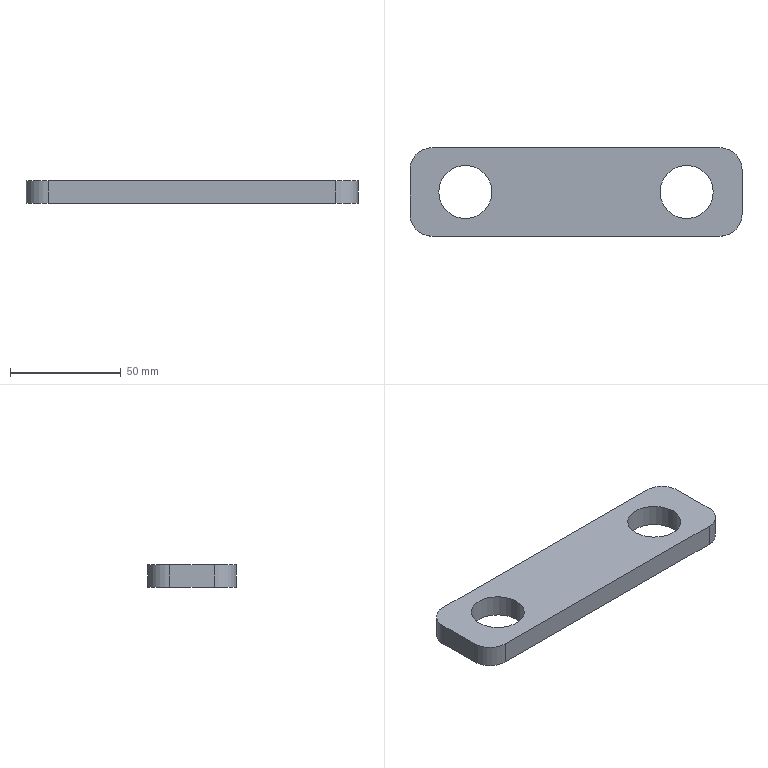Part | SolidWorks | features Extrusion 1, Fillet 1 | 1 solid | 14 faces | box 150 x 40 x 10 mm | volume 50094 mm3 | cylinder 8 | plane 6 | commonest cylinder face diameters 20 x4 24 x4
STEP:
#1=CARTESIAN_POINT('',(-62.,0.,10.));
#2=VERTEX_POINT('',#1);
#3=CARTESIAN_POINT('',(-38.,0.,10.));
#4=VERTEX_POINT('',#3);
#5=CARTESIAN_POINT('',(-50.,0.,10.));
#6=DIRECTION('',(0.,0.,1.));
#7=DIRECTION('',(1.,0.,0.));
#8=AXIS2_PLACEMENT_3D('',#5,#6,#7);
#9=CIRCLE('',#8,12.);
#10=EDGE_CURVE('',#2,#4,#9,.T.);
#11=ORIENTED_EDGE('',*,*,#10,.T.);
#12=CARTESIAN_POINT('',(-38.,0.,0.));
#13=VERTEX_POINT('',#12);
#14=CARTESIAN_POINT('',(-38.,0.,10.));
#15=DIRECTION('',(0.,0.,-1.));
#16=VECTOR('',#15,1000.);
#17=LINE('',#14,#16);
#18=EDGE_CURVE('',#4,#13,#17,.T.);
#19=ORIENTED_EDGE('',*,*,#18,.T.);
#20=CARTESIAN_POINT('',(-62.,0.,0.));
#21=VERTEX_POINT('',#20);
#22=CARTESIAN_POINT('',(-50.,0.,0.));
#23=DIRECTION('',(0.,0.,1.));
#24=DIRECTION('',(1.,0.,0.));
#25=AXIS2_PLACEMENT_3D('',#22,#23,#24);
#26=CIRCLE('',#25,12.);
#27=EDGE_CURVE('',#21,#13,#26,.T.);
#28=ORIENTED_EDGE('',*,*,#27,.F.);
#29=CARTESIAN_POINT('',(-62.,0.,10.));
#30=DIRECTION('',(0.,0.,-1.));
#31=VECTOR('',#30,1000.);
#32=LINE('',#29,#31);
#33=EDGE_CURVE('',#2,#21,#32,.T.);
#34=ORIENTED_EDGE('',*,*,#33,.F.);
#35=EDGE_LOOP('',(#11,#19,#28,#34));
#36=FACE_OUTER_BOUND('',#35,.T.);
#37=CARTESIAN_POINT('',(-50.,0.,10.));
#38=DIRECTION('',(0.,0.,-1.));
#39=DIRECTION('',(-1.,0.,0.));
#40=AXIS2_PLACEMENT_3D('',#37,#38,#39);
#41=CYLINDRICAL_SURFACE('',#40,12.);
#42=ADVANCED_FACE('',(#36),#41,.F.);
#43=CARTESIAN_POINT('',(38.,0.,10.));
#44=VERTEX_POINT('',#43);
#45=CARTESIAN_POINT('',(62.,0.,10.));
#46=VERTEX_POINT('',#45);
#47=CARTESIAN_POINT('',(50.,0.,10.));
#48=DIRECTION('',(0.,0.,1.));
#49=DIRECTION('',(1.,0.,0.));
#50=AXIS2_PLACEMENT_3D('',#47,#48,#49);
#51=CIRCLE('',#50,12.);
#52=EDGE_CURVE('',#44,#46,#51,.T.);
#53=ORIENTED_EDGE('',*,*,#52,.T.);
#54=CARTESIAN_POINT('',(62.,0.,0.));
#55=VERTEX_POINT('',#54);
#56=CARTESIAN_POINT('',(62.,0.,10.));
#57=DIRECTION('',(0.,0.,-1.));
#58=VECTOR('',#57,1000.);
#59=LINE('',#56,#58);
#60=EDGE_CURVE('',#46,#55,#59,.T.);
#61=ORIENTED_EDGE('',*,*,#60,.T.);
#62=CARTESIAN_POINT('',(38.,0.,0.));
#63=VERTEX_POINT('',#62);
#64=CARTESIAN_POINT('',(50.,0.,0.));
#65=DIRECTION('',(0.,0.,1.));
#66=DIRECTION('',(1.,0.,0.));
#67=AXIS2_PLACEMENT_3D('',#64,#65,#66);
#68=CIRCLE('',#67,12.);
#69=EDGE_CURVE('',#63,#55,#68,.T.);
#70=ORIENTED_EDGE('',*,*,#69,.F.);
#71=CARTESIAN_POINT('',(38.,0.,10.));
#72=DIRECTION('',(0.,0.,-1.));
#73=VECTOR('',#72,1000.);
#74=LINE('',#71,#73);
#75=EDGE_CURVE('',#44,#63,#74,.T.);
#76=ORIENTED_EDGE('',*,*,#75,.F.);
#77=EDGE_LOOP('',(#53,#61,#70,#76));
#78=FACE_OUTER_BOUND('',#77,.T.);
#79=CARTESIAN_POINT('',(50.,0.,10.));
#80=DIRECTION('',(0.,0.,-1.));
#81=DIRECTION('',(-1.,0.,0.));
#82=AXIS2_PLACEMENT_3D('',#79,#80,#81);
#83=CYLINDRICAL_SURFACE('',#82,12.);
#84=ADVANCED_FACE('',(#78),#83,.F.);
#85=ORIENTED_EDGE('',*,*,#52,.F.);
#86=CARTESIAN_POINT('',(50.,0.,10.));
#87=DIRECTION('',(0.,0.,1.));
#88=DIRECTION('',(1.,0.,0.));
#89=AXIS2_PLACEMENT_3D('',#86,#87,#88);
#90=CIRCLE('',#89,12.);
#91=EDGE_CURVE('',#46,#44,#90,.T.);
#92=ORIENTED_EDGE('',*,*,#91,.F.);
#93=EDGE_LOOP('',(#85,#92));
#94=FACE_BOUND('',#93,.T.);
#95=CARTESIAN_POINT('',(75.,-10.,10.));
#96=VERTEX_POINT('',#95);
#97=CARTESIAN_POINT('',(75.,10.,10.));
#98=VERTEX_POINT('',#97);
#99=CARTESIAN_POINT('',(75.,20.,10.));
#100=DIRECTION('',(0.,1.,0.));
#101=VECTOR('',#100,1000.);
#102=LINE('',#99,#101);
#103=EDGE_CURVE('',#96,#98,#102,.T.);
#104=ORIENTED_EDGE('',*,*,#103,.T.);
#105=CARTESIAN_POINT('',(65.,20.,10.));
#106=VERTEX_POINT('',#105);
#107=CARTESIAN_POINT('',(65.,10.,10.));
#108=DIRECTION('',(0.,0.,1.));
#109=DIRECTION('',(1.,0.,0.));
#110=AXIS2_PLACEMENT_3D('',#107,#108,#109);
#111=CIRCLE('',#110,10.);
#112=EDGE_CURVE('',#98,#106,#111,.T.);
#113=ORIENTED_EDGE('',*,*,#112,.T.);
#114=CARTESIAN_POINT('',(-65.,20.,10.));
#115=VERTEX_POINT('',#114);
#116=CARTESIAN_POINT('',(-75.,20.,10.));
#117=DIRECTION('',(-1.,0.,0.));
#118=VECTOR('',#117,1000.);
#119=LINE('',#116,#118);
#120=EDGE_CURVE('',#106,#115,#119,.T.);
#121=ORIENTED_EDGE('',*,*,#120,.T.);
#122=CARTESIAN_POINT('',(-75.,10.,10.));
#123=VERTEX_POINT('',#122);
#124=CARTESIAN_POINT('',(-65.,10.,10.));
#125=DIRECTION('',(0.,0.,1.));
#126=DIRECTION('',(1.,0.,0.));
#127=AXIS2_PLACEMENT_3D('',#124,#125,#126);
#128=CIRCLE('',#127,10.);
#129=EDGE_CURVE('',#115,#123,#128,.T.);
#130=ORIENTED_EDGE('',*,*,#129,.T.);
#131=CARTESIAN_POINT('',(-75.,-10.,10.));
#132=VERTEX_POINT('',#131);
#133=CARTESIAN_POINT('',(-75.,20.,10.));
#134=DIRECTION('',(0.,-1.,0.));
#135=VECTOR('',#134,1000.);
#136=LINE('',#133,#135);
#137=EDGE_CURVE('',#123,#132,#136,.T.);
#138=ORIENTED_EDGE('',*,*,#137,.T.);
#139=CARTESIAN_POINT('',(-65.,-20.,10.));
#140=VERTEX_POINT('',#139);
#141=CARTESIAN_POINT('',(-65.,-10.,10.));
#142=DIRECTION('',(0.,0.,1.));
#143=DIRECTION('',(1.,0.,0.));
#144=AXIS2_PLACEMENT_3D('',#141,#142,#143);
#145=CIRCLE('',#144,10.);
#146=EDGE_CURVE('',#132,#140,#145,.T.);
#147=ORIENTED_EDGE('',*,*,#146,.T.);
#148=CARTESIAN_POINT('',(65.,-20.,10.));
#149=VERTEX_POINT('',#148);
#150=CARTESIAN_POINT('',(-75.,-20.,10.));
#151=DIRECTION('',(1.,0.,0.));
#152=VECTOR('',#151,1000.);
#153=LINE('',#150,#152);
#154=EDGE_CURVE('',#140,#149,#153,.T.);
#155=ORIENTED_EDGE('',*,*,#154,.T.);
#156=CARTESIAN_POINT('',(65.,-10.,10.));
#157=DIRECTION('',(0.,0.,1.));
#158=DIRECTION('',(1.,0.,0.));
#159=AXIS2_PLACEMENT_3D('',#156,#157,#158);
#160=CIRCLE('',#159,10.);
#161=EDGE_CURVE('',#149,#96,#160,.T.);
#162=ORIENTED_EDGE('',*,*,#161,.T.);
#163=EDGE_LOOP('',(#104,#113,#121,#130,#138,#147,#155,#162));
#164=FACE_OUTER_BOUND('',#163,.T.);
#165=ORIENTED_EDGE('',*,*,#10,.F.);
#166=CARTESIAN_POINT('',(-50.,0.,10.));
#167=DIRECTION('',(0.,0.,1.));
#168=DIRECTION('',(1.,0.,0.));
#169=AXIS2_PLACEMENT_3D('',#166,#167,#168);
#170=CIRCLE('',#169,12.);
#171=EDGE_CURVE('',#4,#2,#170,.T.);
#172=ORIENTED_EDGE('',*,*,#171,.F.);
#173=EDGE_LOOP('',(#165,#172));
#174=FACE_BOUND('',#173,.T.);
#175=CARTESIAN_POINT('',(0.,0.,10.));
#176=DIRECTION('',(0.,0.,1.));
#177=DIRECTION('',(1.,0.,0.));
#178=AXIS2_PLACEMENT_3D('',#175,#176,#177);
#179=PLANE('',#178);
#180=ADVANCED_FACE('',(#94,#164,#174),#179,.T.);
#181=CARTESIAN_POINT('',(65.,20.,0.));
#182=VERTEX_POINT('',#181);
#183=CARTESIAN_POINT('',(-65.,20.,0.));
#184=VERTEX_POINT('',#183);
#185=CARTESIAN_POINT('',(-75.,20.,0.));
#186=DIRECTION('',(-1.,0.,0.));
#187=VECTOR('',#186,1000.);
#188=LINE('',#185,#187);
#189=EDGE_CURVE('',#182,#184,#188,.T.);
#190=ORIENTED_EDGE('',*,*,#189,.F.);
#191=CARTESIAN_POINT('',(75.,10.,0.));
#192=VERTEX_POINT('',#191);
#193=CARTESIAN_POINT('',(65.,10.,0.));
#194=DIRECTION('',(0.,0.,-1.));
#195=DIRECTION('',(1.,0.,0.));
#196=AXIS2_PLACEMENT_3D('',#193,#194,#195);
#197=CIRCLE('',#196,10.);
#198=EDGE_CURVE('',#182,#192,#197,.T.);
#199=ORIENTED_EDGE('',*,*,#198,.T.);
#200=CARTESIAN_POINT('',(75.,-10.,0.));
#201=VERTEX_POINT('',#200);
#202=CARTESIAN_POINT('',(75.,20.,0.));
#203=DIRECTION('',(0.,1.,0.));
#204=VECTOR('',#203,1000.);
#205=LINE('',#202,#204);
#206=EDGE_CURVE('',#201,#192,#205,.T.);
#207=ORIENTED_EDGE('',*,*,#206,.F.);
#208=CARTESIAN_POINT('',(65.,-20.,0.));
#209=VERTEX_POINT('',#208);
#210=CARTESIAN_POINT('',(65.,-10.,0.));
#211=DIRECTION('',(0.,0.,-1.));
#212=DIRECTION('',(1.,0.,0.));
#213=AXIS2_PLACEMENT_3D('',#210,#211,#212);
#214=CIRCLE('',#213,10.);
#215=EDGE_CURVE('',#201,#209,#214,.T.);
#216=ORIENTED_EDGE('',*,*,#215,.T.);
#217=CARTESIAN_POINT('',(-65.,-20.,0.));
#218=VERTEX_POINT('',#217);
#219=CARTESIAN_POINT('',(-75.,-20.,0.));
#220=DIRECTION('',(1.,0.,0.));
#221=VECTOR('',#220,1000.);
#222=LINE('',#219,#221);
#223=EDGE_CURVE('',#218,#209,#222,.T.);
#224=ORIENTED_EDGE('',*,*,#223,.F.);
#225=CARTESIAN_POINT('',(-75.,-10.,0.));
#226=VERTEX_POINT('',#225);
#227=CARTESIAN_POINT('',(-65.,-10.,0.));
#228=DIRECTION('',(0.,0.,-1.));
#229=DIRECTION('',(1.,0.,0.));
#230=AXIS2_PLACEMENT_3D('',#227,#228,#229);
#231=CIRCLE('',#230,10.);
#232=EDGE_CURVE('',#218,#226,#231,.T.);
#233=ORIENTED_EDGE('',*,*,#232,.T.);
#234=CARTESIAN_POINT('',(-75.,10.,0.));
#235=VERTEX_POINT('',#234);
#236=CARTESIAN_POINT('',(-75.,20.,0.));
#237=DIRECTION('',(0.,-1.,0.));
#238=VECTOR('',#237,1000.);
#239=LINE('',#236,#238);
#240=EDGE_CURVE('',#235,#226,#239,.T.);
#241=ORIENTED_EDGE('',*,*,#240,.F.);
#242=CARTESIAN_POINT('',(-65.,10.,0.));
#243=DIRECTION('',(0.,0.,-1.));
#244=DIRECTION('',(1.,0.,0.));
#245=AXIS2_PLACEMENT_3D('',#242,#243,#244);
#246=CIRCLE('',#245,10.);
#247=EDGE_CURVE('',#235,#184,#246,.T.);
#248=ORIENTED_EDGE('',*,*,#247,.T.);
#249=EDGE_LOOP('',(#190,#199,#207,#216,#224,#233,#241,#248));
#250=FACE_OUTER_BOUND('',#249,.T.);
#251=ORIENTED_EDGE('',*,*,#69,.T.);
#252=CARTESIAN_POINT('',(50.,0.,0.));
#253=DIRECTION('',(0.,0.,1.));
#254=DIRECTION('',(1.,0.,0.));
#255=AXIS2_PLACEMENT_3D('',#252,#253,#254);
#256=CIRCLE('',#255,12.);
#257=EDGE_CURVE('',#55,#63,#256,.T.);
#258=ORIENTED_EDGE('',*,*,#257,.T.);
#259=EDGE_LOOP('',(#251,#258));
#260=FACE_BOUND('',#259,.T.);
#261=ORIENTED_EDGE('',*,*,#27,.T.);
#262=CARTESIAN_POINT('',(-50.,0.,0.));
#263=DIRECTION('',(0.,0.,1.));
#264=DIRECTION('',(1.,0.,0.));
#265=AXIS2_PLACEMENT_3D('',#262,#263,#264);
#266=CIRCLE('',#265,12.);
#267=EDGE_CURVE('',#13,#21,#266,.T.);
#268=ORIENTED_EDGE('',*,*,#267,.T.);
#269=EDGE_LOOP('',(#261,#268));
#270=FACE_BOUND('',#269,.T.);
#271=CARTESIAN_POINT('',(0.,0.,0.));
#272=DIRECTION('',(0.,0.,1.));
#273=DIRECTION('',(1.,0.,0.));
#274=AXIS2_PLACEMENT_3D('',#271,#272,#273);
#275=PLANE('',#274);
#276=ADVANCED_FACE('',(#250,#260,#270),#275,.F.);
#277=ORIENTED_EDGE('',*,*,#206,.T.);
#278=CARTESIAN_POINT('',(75.,10.,10.));
#279=DIRECTION('',(0.,0.,1.));
#280=VECTOR('',#279,1000.);
#281=LINE('',#278,#280);
#282=EDGE_CURVE('',#192,#98,#281,.T.);
#283=ORIENTED_EDGE('',*,*,#282,.T.);
#284=ORIENTED_EDGE('',*,*,#103,.F.);
#285=CARTESIAN_POINT('',(75.,-10.,10.));
#286=DIRECTION('',(0.,0.,-1.));
#287=VECTOR('',#286,1000.);
#288=LINE('',#285,#287);
#289=EDGE_CURVE('',#96,#201,#288,.T.);
#290=ORIENTED_EDGE('',*,*,#289,.T.);
#291=EDGE_LOOP('',(#277,#283,#284,#290));
#292=FACE_OUTER_BOUND('',#291,.T.);
#293=CARTESIAN_POINT('',(75.,20.,10.));
#294=DIRECTION('',(-1.,0.,0.));
#295=DIRECTION('',(0.,0.,1.));
#296=AXIS2_PLACEMENT_3D('',#293,#294,#295);
#297=PLANE('',#296);
#298=ADVANCED_FACE('',(#292),#297,.F.);
#299=ORIENTED_EDGE('',*,*,#120,.F.);
#300=CARTESIAN_POINT('',(65.,20.,10.));
#301=DIRECTION('',(0.,0.,-1.));
#302=VECTOR('',#301,1000.);
#303=LINE('',#300,#302);
#304=EDGE_CURVE('',#106,#182,#303,.T.);
#305=ORIENTED_EDGE('',*,*,#304,.T.);
#306=ORIENTED_EDGE('',*,*,#189,.T.);
#307=CARTESIAN_POINT('',(-65.,20.,10.));
#308=DIRECTION('',(0.,0.,1.));
#309=VECTOR('',#308,1000.);
#310=LINE('',#307,#309);
#311=EDGE_CURVE('',#184,#115,#310,.T.);
#312=ORIENTED_EDGE('',*,*,#311,.T.);
#313=EDGE_LOOP('',(#299,#305,#306,#312));
#314=FACE_OUTER_BOUND('',#313,.T.);
#315=CARTESIAN_POINT('',(-75.,20.,10.));
#316=DIRECTION('',(0.,-1.,0.));
#317=DIRECTION('',(0.,0.,-1.));
#318=AXIS2_PLACEMENT_3D('',#315,#316,#317);
#319=PLANE('',#318);
#320=ADVANCED_FACE('',(#314),#319,.F.);
#321=ORIENTED_EDGE('',*,*,#240,.T.);
#322=CARTESIAN_POINT('',(-75.,-10.,10.));
#323=DIRECTION('',(0.,0.,1.));
#324=VECTOR('',#323,1000.);
#325=LINE('',#322,#324);
#326=EDGE_CURVE('',#226,#132,#325,.T.);
#327=ORIENTED_EDGE('',*,*,#326,.T.);
#328=ORIENTED_EDGE('',*,*,#137,.F.);
#329=CARTESIAN_POINT('',(-75.,10.,10.));
#330=DIRECTION('',(0.,0.,-1.));
#331=VECTOR('',#330,1000.);
#332=LINE('',#329,#331);
#333=EDGE_CURVE('',#123,#235,#332,.T.);
#334=ORIENTED_EDGE('',*,*,#333,.T.);
#335=EDGE_LOOP('',(#321,#327,#328,#334));
#336=FACE_OUTER_BOUND('',#335,.T.);
#337=CARTESIAN_POINT('',(-75.,20.,10.));
#338=DIRECTION('',(1.,0.,0.));
#339=DIRECTION('',(0.,0.,-1.));
#340=AXIS2_PLACEMENT_3D('',#337,#338,#339);
#341=PLANE('',#340);
#342=ADVANCED_FACE('',(#336),#341,.F.);
#343=ORIENTED_EDGE('',*,*,#154,.F.);
#344=CARTESIAN_POINT('',(-65.,-20.,10.));
#345=DIRECTION('',(0.,0.,-1.));
#346=VECTOR('',#345,1000.);
#347=LINE('',#344,#346);
#348=EDGE_CURVE('',#140,#218,#347,.T.);
#349=ORIENTED_EDGE('',*,*,#348,.T.);
#350=ORIENTED_EDGE('',*,*,#223,.T.);
#351=CARTESIAN_POINT('',(65.,-20.,10.));
#352=DIRECTION('',(0.,0.,1.));
#353=VECTOR('',#352,1000.);
#354=LINE('',#351,#353);
#355=EDGE_CURVE('',#209,#149,#354,.T.);
#356=ORIENTED_EDGE('',*,*,#355,.T.);
#357=EDGE_LOOP('',(#343,#349,#350,#356));
#358=FACE_OUTER_BOUND('',#357,.T.);
#359=CARTESIAN_POINT('',(-75.,-20.,10.));
#360=DIRECTION('',(0.,1.,0.));
#361=DIRECTION('',(0.,0.,1.));
#362=AXIS2_PLACEMENT_3D('',#359,#360,#361);
#363=PLANE('',#362);
#364=ADVANCED_FACE('',(#358),#363,.F.);
#365=ORIENTED_EDGE('',*,*,#60,.F.);
#366=ORIENTED_EDGE('',*,*,#91,.T.);
#367=ORIENTED_EDGE('',*,*,#75,.T.);
#368=ORIENTED_EDGE('',*,*,#257,.F.);
#369=EDGE_LOOP('',(#365,#366,#367,#368));
#370=FACE_OUTER_BOUND('',#369,.T.);
#371=CARTESIAN_POINT('',(50.,0.,10.));
#372=DIRECTION('',(0.,0.,-1.));
#373=DIRECTION('',(-1.,0.,0.));
#374=AXIS2_PLACEMENT_3D('',#371,#372,#373);
#375=CYLINDRICAL_SURFACE('',#374,12.);
#376=ADVANCED_FACE('',(#370),#375,.F.);
#377=ORIENTED_EDGE('',*,*,#18,.F.);
#378=ORIENTED_EDGE('',*,*,#171,.T.);
#379=ORIENTED_EDGE('',*,*,#33,.T.);
#380=ORIENTED_EDGE('',*,*,#267,.F.);
#381=EDGE_LOOP('',(#377,#378,#379,#380));
#382=FACE_OUTER_BOUND('',#381,.T.);
#383=CARTESIAN_POINT('',(-50.,0.,10.));
#384=DIRECTION('',(0.,0.,-1.));
#385=DIRECTION('',(-1.,0.,0.));
#386=AXIS2_PLACEMENT_3D('',#383,#384,#385);
#387=CYLINDRICAL_SURFACE('',#386,12.);
#388=ADVANCED_FACE('',(#382),#387,.F.);
#389=ORIENTED_EDGE('',*,*,#112,.F.);
#390=ORIENTED_EDGE('',*,*,#282,.F.);
#391=ORIENTED_EDGE('',*,*,#198,.F.);
#392=ORIENTED_EDGE('',*,*,#304,.F.);
#393=EDGE_LOOP('',(#389,#390,#391,#392));
#394=FACE_OUTER_BOUND('',#393,.T.);
#395=CARTESIAN_POINT('',(65.,10.,10.));
#396=DIRECTION('',(0.,0.,-1.));
#397=DIRECTION('',(-1.,0.,0.));
#398=AXIS2_PLACEMENT_3D('',#395,#396,#397);
#399=CYLINDRICAL_SURFACE('',#398,10.);
#400=ADVANCED_FACE('',(#394),#399,.T.);
#401=ORIENTED_EDGE('',*,*,#146,.F.);
#402=ORIENTED_EDGE('',*,*,#326,.F.);
#403=ORIENTED_EDGE('',*,*,#232,.F.);
#404=ORIENTED_EDGE('',*,*,#348,.F.);
#405=EDGE_LOOP('',(#401,#402,#403,#404));
#406=FACE_OUTER_BOUND('',#405,.T.);
#407=CARTESIAN_POINT('',(-65.,-10.,10.));
#408=DIRECTION('',(0.,0.,-1.));
#409=DIRECTION('',(-1.,0.,0.));
#410=AXIS2_PLACEMENT_3D('',#407,#408,#409);
#411=CYLINDRICAL_SURFACE('',#410,10.);
#412=ADVANCED_FACE('',(#406),#411,.T.);
#413=ORIENTED_EDGE('',*,*,#129,.F.);
#414=ORIENTED_EDGE('',*,*,#311,.F.);
#415=ORIENTED_EDGE('',*,*,#247,.F.);
#416=ORIENTED_EDGE('',*,*,#333,.F.);
#417=EDGE_LOOP('',(#413,#414,#415,#416));
#418=FACE_OUTER_BOUND('',#417,.T.);
#419=CARTESIAN_POINT('',(-65.,10.,10.));
#420=DIRECTION('',(0.,0.,-1.));
#421=DIRECTION('',(-1.,0.,0.));
#422=AXIS2_PLACEMENT_3D('',#419,#420,#421);
#423=CYLINDRICAL_SURFACE('',#422,10.);
#424=ADVANCED_FACE('',(#418),#423,.T.);
#425=ORIENTED_EDGE('',*,*,#161,.F.);
#426=ORIENTED_EDGE('',*,*,#355,.F.);
#427=ORIENTED_EDGE('',*,*,#215,.F.);
#428=ORIENTED_EDGE('',*,*,#289,.F.);
#429=EDGE_LOOP('',(#425,#426,#427,#428));
#430=FACE_OUTER_BOUND('',#429,.T.);
#431=CARTESIAN_POINT('',(65.,-10.,10.));
#432=DIRECTION('',(0.,0.,-1.));
#433=DIRECTION('',(-1.,0.,0.));
#434=AXIS2_PLACEMENT_3D('',#431,#432,#433);
#435=CYLINDRICAL_SURFACE('',#434,10.);
#436=ADVANCED_FACE('',(#430),#435,.T.);
#437=CLOSED_SHELL('',(#42,#84,#180,#276,#298,#320,#342,#364,#376,#388,#400,#412,#424,#436));
#438=MANIFOLD_SOLID_BREP('',#437);
#439=CARTESIAN_POINT('',(0.,0.,0.));
#440=DIRECTION('',(0.,0.,1.));
#441=DIRECTION('',(1.,0.,0.));
#442=AXIS2_PLACEMENT_3D('',#439,#440,#441);
#443=(LENGTH_UNIT()NAMED_UNIT(*)SI_UNIT(.MILLI.,.METRE.));
#444=UNCERTAINTY_MEASURE_WITH_UNIT(LENGTH_MEASURE(0.00001),#443,'','');
#445=(NAMED_UNIT(*)PLANE_ANGLE_UNIT()SI_UNIT($,.RADIAN.));
#446=(NAMED_UNIT(*)SI_UNIT($,.STERADIAN.)SOLID_ANGLE_UNIT());
#447=(GEOMETRIC_REPRESENTATION_CONTEXT(3)GLOBAL_UNCERTAINTY_ASSIGNED_CONTEXT((#444))GLOBAL_UNIT_ASSIGNED_CONTEXT((#443,#445,#446))REPRESENTATION_CONTEXT('',''));
#448=ADVANCED_BREP_SHAPE_REPRESENTATION('',(#438,#442),#447);